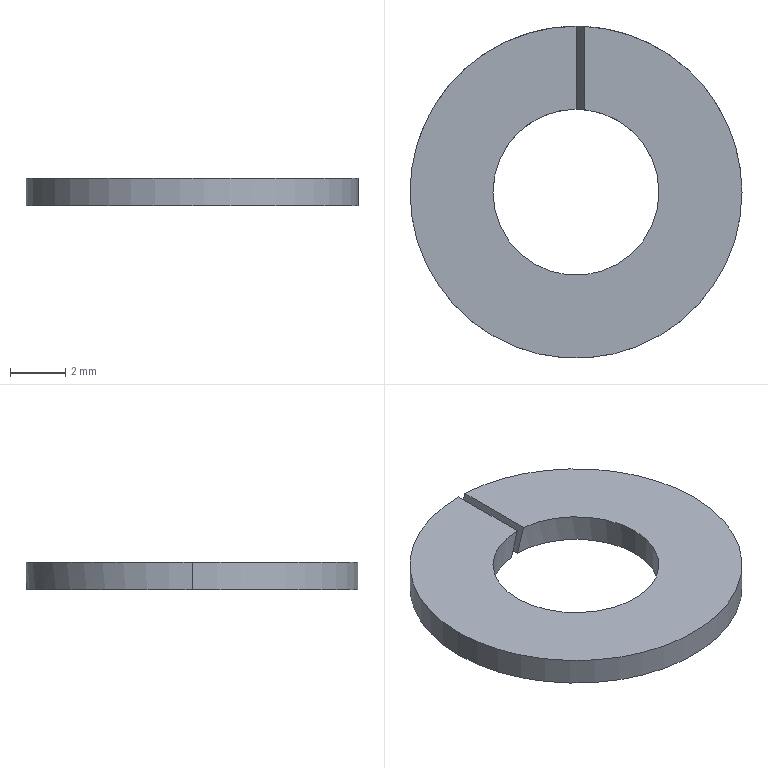Part | NX | features BREP 1 | 1 solid | 10 faces | box 12 x 12 x 1 mm | volume 83.879 mm3 | cylinder 6 | plane 4 | commonest cylinder face diameters 6 x3 12 x3
STEP:
#1=CARTESIAN_POINT('',(-3.,0.,-1.));
#2=VERTEX_POINT('',#1);
#3=CARTESIAN_POINT('',(3.,0.,-1.));
#4=VERTEX_POINT('',#3);
#5=CARTESIAN_POINT('',(0.,0.,-1.));
#6=DIRECTION('',(0.,0.,1.));
#7=DIRECTION('',(1.,0.,0.));
#8=AXIS2_PLACEMENT_3D('',#5,#6,#7);
#9=CIRCLE('',#8,3.);
#10=EDGE_CURVE('',#2,#4,#9,.T.);
#11=ORIENTED_EDGE('',*,*,#10,.F.);
#12=CARTESIAN_POINT('',(-3.,0.,0.));
#13=VERTEX_POINT('',#12);
#14=CARTESIAN_POINT('',(-3.,0.,-1.));
#15=DIRECTION('',(0.,0.,1.));
#16=VECTOR('',#15,1000.);
#17=LINE('',#14,#16);
#18=EDGE_CURVE('',#2,#13,#17,.T.);
#19=ORIENTED_EDGE('',*,*,#18,.T.);
#20=CARTESIAN_POINT('',(3.,0.,0.));
#21=VERTEX_POINT('',#20);
#22=CARTESIAN_POINT('',(0.,0.,0.));
#23=DIRECTION('',(0.,0.,1.));
#24=DIRECTION('',(1.,0.,0.));
#25=AXIS2_PLACEMENT_3D('',#22,#23,#24);
#26=CIRCLE('',#25,3.);
#27=EDGE_CURVE('',#13,#21,#26,.T.);
#28=ORIENTED_EDGE('',*,*,#27,.T.);
#29=CARTESIAN_POINT('',(3.,0.,-1.));
#30=DIRECTION('',(0.,0.,1.));
#31=VECTOR('',#30,1000.);
#32=LINE('',#29,#31);
#33=EDGE_CURVE('',#4,#21,#32,.T.);
#34=ORIENTED_EDGE('',*,*,#33,.F.);
#35=EDGE_LOOP('',(#11,#19,#28,#34));
#36=FACE_BOUND('',#35,.T.);
#37=CARTESIAN_POINT('',(0.,0.,-1.));
#38=DIRECTION('',(0.,0.,1.));
#39=DIRECTION('',(-1.,0.,0.));
#40=AXIS2_PLACEMENT_3D('',#37,#38,#39);
#41=CYLINDRICAL_SURFACE('',#40,3.);
#42=ADVANCED_FACE('',(#36),#41,.F.);
#43=CARTESIAN_POINT('',(0.,3.,-1.));
#44=VERTEX_POINT('',#43);
#45=CARTESIAN_POINT('',(0.,0.,-1.));
#46=DIRECTION('',(0.,0.,1.));
#47=DIRECTION('',(1.,0.,0.));
#48=AXIS2_PLACEMENT_3D('',#45,#46,#47);
#49=CIRCLE('',#48,3.);
#50=EDGE_CURVE('',#4,#44,#49,.T.);
#51=ORIENTED_EDGE('',*,*,#50,.F.);
#52=ORIENTED_EDGE('',*,*,#33,.T.);
#53=CARTESIAN_POINT('',(0.3145,2.983,0.));
#54=VERTEX_POINT('',#53);
#55=CARTESIAN_POINT('',(0.,0.,0.));
#56=DIRECTION('',(0.,0.,1.));
#57=DIRECTION('',(1.,0.,0.));
#58=AXIS2_PLACEMENT_3D('',#55,#56,#57);
#59=CIRCLE('',#58,3.);
#60=EDGE_CURVE('',#21,#54,#59,.T.);
#61=ORIENTED_EDGE('',*,*,#60,.T.);
#62=CARTESIAN_POINT('',(0.,3.,-1.));
#63=CARTESIAN_POINT('',(0.1051,3.,-0.6659));
#64=CARTESIAN_POINT('',(0.21,2.994,-0.3323));
#65=CARTESIAN_POINT('',(0.3145,2.983,0.));
#66=(BOUNDED_CURVE()B_SPLINE_CURVE(3,(#62,#63,#64,#65),.UNSPECIFIED.,.F.,.F.)B_SPLINE_CURVE_WITH_KNOTS((4,4),(0.,1.),.PIECEWISE_BEZIER_KNOTS.)CURVE()GEOMETRIC_REPRESENTATION_ITEM()RATIONAL_B_SPLINE_CURVE((1.,0.9991,0.9991,1.))REPRESENTATION_ITEM(''));
#67=EDGE_CURVE('',#44,#54,#66,.T.);
#68=ORIENTED_EDGE('',*,*,#67,.F.);
#69=EDGE_LOOP('',(#51,#52,#61,#68));
#70=FACE_BOUND('',#69,.T.);
#71=CARTESIAN_POINT('',(0.,0.,-1.));
#72=DIRECTION('',(0.,0.,1.));
#73=DIRECTION('',(-1.,0.,0.));
#74=AXIS2_PLACEMENT_3D('',#71,#72,#73);
#75=CYLINDRICAL_SURFACE('',#74,3.);
#76=ADVANCED_FACE('',(#70),#75,.F.);
#77=CARTESIAN_POINT('',(-0.3145,5.992,-1.));
#78=VERTEX_POINT('',#77);
#79=CARTESIAN_POINT('',(-6.,0.,-1.));
#80=VERTEX_POINT('',#79);
#81=CARTESIAN_POINT('',(0.,0.,-1.));
#82=DIRECTION('',(0.,0.,1.));
#83=DIRECTION('',(1.,0.,0.));
#84=AXIS2_PLACEMENT_3D('',#81,#82,#83);
#85=CIRCLE('',#84,6.);
#86=EDGE_CURVE('',#78,#80,#85,.T.);
#87=ORIENTED_EDGE('',*,*,#86,.T.);
#88=CARTESIAN_POINT('',(-6.,0.,0.));
#89=VERTEX_POINT('',#88);
#90=CARTESIAN_POINT('',(-6.,0.,-1.));
#91=DIRECTION('',(0.,0.,1.));
#92=VECTOR('',#91,1000.);
#93=LINE('',#90,#92);
#94=EDGE_CURVE('',#80,#89,#93,.T.);
#95=ORIENTED_EDGE('',*,*,#94,.T.);
#96=CARTESIAN_POINT('',(0.,6.,0.));
#97=VERTEX_POINT('',#96);
#98=CARTESIAN_POINT('',(0.,0.,0.));
#99=DIRECTION('',(0.,0.,1.));
#100=DIRECTION('',(1.,0.,0.));
#101=AXIS2_PLACEMENT_3D('',#98,#99,#100);
#102=CIRCLE('',#101,6.);
#103=EDGE_CURVE('',#97,#89,#102,.T.);
#104=ORIENTED_EDGE('',*,*,#103,.F.);
#105=CARTESIAN_POINT('',(0.,6.,0.));
#106=CARTESIAN_POINT('',(-0.1049,6.,-0.3335));
#107=CARTESIAN_POINT('',(-0.2097,5.997,-0.6669));
#108=CARTESIAN_POINT('',(-0.3145,5.992,-1.));
#109=(BOUNDED_CURVE()B_SPLINE_CURVE(3,(#105,#106,#107,#108),.UNSPECIFIED.,.F.,.F.)B_SPLINE_CURVE_WITH_KNOTS((4,4),(0.,1.),.PIECEWISE_BEZIER_KNOTS.)CURVE()GEOMETRIC_REPRESENTATION_ITEM()RATIONAL_B_SPLINE_CURVE((1.,0.9998,0.9998,1.))REPRESENTATION_ITEM(''));
#110=EDGE_CURVE('',#97,#78,#109,.T.);
#111=ORIENTED_EDGE('',*,*,#110,.T.);
#112=EDGE_LOOP('',(#87,#95,#104,#111));
#113=FACE_BOUND('',#112,.T.);
#114=CARTESIAN_POINT('',(0.,0.,-1.));
#115=DIRECTION('',(0.,0.,1.));
#116=DIRECTION('',(-1.,0.,0.));
#117=AXIS2_PLACEMENT_3D('',#114,#115,#116);
#118=CYLINDRICAL_SURFACE('',#117,6.);
#119=ADVANCED_FACE('',(#113),#118,.T.);
#120=ORIENTED_EDGE('',*,*,#94,.F.);
#121=CARTESIAN_POINT('',(6.,0.,-1.));
#122=VERTEX_POINT('',#121);
#123=CARTESIAN_POINT('',(0.,0.,-1.));
#124=DIRECTION('',(0.,0.,1.));
#125=DIRECTION('',(1.,0.,0.));
#126=AXIS2_PLACEMENT_3D('',#123,#124,#125);
#127=CIRCLE('',#126,6.);
#128=EDGE_CURVE('',#80,#122,#127,.T.);
#129=ORIENTED_EDGE('',*,*,#128,.T.);
#130=CARTESIAN_POINT('',(6.,0.,0.));
#131=VERTEX_POINT('',#130);
#132=CARTESIAN_POINT('',(6.,0.,-1.));
#133=DIRECTION('',(0.,0.,1.));
#134=VECTOR('',#133,1000.);
#135=LINE('',#132,#134);
#136=EDGE_CURVE('',#122,#131,#135,.T.);
#137=ORIENTED_EDGE('',*,*,#136,.T.);
#138=CARTESIAN_POINT('',(0.,0.,0.));
#139=DIRECTION('',(0.,0.,1.));
#140=DIRECTION('',(1.,0.,0.));
#141=AXIS2_PLACEMENT_3D('',#138,#139,#140);
#142=CIRCLE('',#141,6.);
#143=EDGE_CURVE('',#89,#131,#142,.T.);
#144=ORIENTED_EDGE('',*,*,#143,.F.);
#145=EDGE_LOOP('',(#120,#129,#137,#144));
#146=FACE_BOUND('',#145,.T.);
#147=CARTESIAN_POINT('',(0.,0.,-1.));
#148=DIRECTION('',(0.,0.,1.));
#149=DIRECTION('',(-1.,0.,0.));
#150=AXIS2_PLACEMENT_3D('',#147,#148,#149);
#151=CYLINDRICAL_SURFACE('',#150,6.);
#152=ADVANCED_FACE('',(#146),#151,.T.);
#153=ORIENTED_EDGE('',*,*,#136,.F.);
#154=CARTESIAN_POINT('',(0.,6.,-1.));
#155=VERTEX_POINT('',#154);
#156=CARTESIAN_POINT('',(0.,0.,-1.));
#157=DIRECTION('',(0.,0.,1.));
#158=DIRECTION('',(1.,0.,0.));
#159=AXIS2_PLACEMENT_3D('',#156,#157,#158);
#160=CIRCLE('',#159,6.);
#161=EDGE_CURVE('',#122,#155,#160,.T.);
#162=ORIENTED_EDGE('',*,*,#161,.T.);
#163=CARTESIAN_POINT('',(0.3145,5.992,0.));
#164=VERTEX_POINT('',#163);
#165=CARTESIAN_POINT('',(0.,6.,-1.));
#166=CARTESIAN_POINT('',(0.1049,6.,-0.6665));
#167=CARTESIAN_POINT('',(0.2097,5.997,-0.3331));
#168=CARTESIAN_POINT('',(0.3145,5.992,0.));
#169=(BOUNDED_CURVE()B_SPLINE_CURVE(3,(#165,#166,#167,#168),.UNSPECIFIED.,.F.,.F.)B_SPLINE_CURVE_WITH_KNOTS((4,4),(0.,1.),.PIECEWISE_BEZIER_KNOTS.)CURVE()GEOMETRIC_REPRESENTATION_ITEM()RATIONAL_B_SPLINE_CURVE((1.,0.9998,0.9998,1.))REPRESENTATION_ITEM(''));
#170=EDGE_CURVE('',#155,#164,#169,.T.);
#171=ORIENTED_EDGE('',*,*,#170,.T.);
#172=CARTESIAN_POINT('',(0.,0.,0.));
#173=DIRECTION('',(0.,0.,1.));
#174=DIRECTION('',(1.,0.,0.));
#175=AXIS2_PLACEMENT_3D('',#172,#173,#174);
#176=CIRCLE('',#175,6.);
#177=EDGE_CURVE('',#131,#164,#176,.T.);
#178=ORIENTED_EDGE('',*,*,#177,.F.);
#179=EDGE_LOOP('',(#153,#162,#171,#178));
#180=FACE_BOUND('',#179,.T.);
#181=CARTESIAN_POINT('',(0.,0.,-1.));
#182=DIRECTION('',(0.,0.,1.));
#183=DIRECTION('',(-1.,0.,0.));
#184=AXIS2_PLACEMENT_3D('',#181,#182,#183);
#185=CYLINDRICAL_SURFACE('',#184,6.);
#186=ADVANCED_FACE('',(#180),#185,.T.);
#187=CARTESIAN_POINT('',(-0.3145,2.983,-1.));
#188=VERTEX_POINT('',#187);
#189=CARTESIAN_POINT('',(-0.3145,6.,-1.));
#190=DIRECTION('',(0.,-1.,0.));
#191=VECTOR('',#190,1000.);
#192=LINE('',#189,#191);
#193=EDGE_CURVE('',#78,#188,#192,.T.);
#194=ORIENTED_EDGE('',*,*,#193,.T.);
#195=CARTESIAN_POINT('',(0.,0.,-1.));
#196=DIRECTION('',(0.,0.,1.));
#197=DIRECTION('',(1.,0.,0.));
#198=AXIS2_PLACEMENT_3D('',#195,#196,#197);
#199=CIRCLE('',#198,3.);
#200=EDGE_CURVE('',#188,#2,#199,.T.);
#201=ORIENTED_EDGE('',*,*,#200,.T.);
#202=ORIENTED_EDGE('',*,*,#10,.T.);
#203=ORIENTED_EDGE('',*,*,#50,.T.);
#204=CARTESIAN_POINT('',(0.,6.,-1.));
#205=DIRECTION('',(0.,-1.,0.));
#206=VECTOR('',#205,1000.);
#207=LINE('',#204,#206);
#208=EDGE_CURVE('',#155,#44,#207,.T.);
#209=ORIENTED_EDGE('',*,*,#208,.F.);
#210=ORIENTED_EDGE('',*,*,#161,.F.);
#211=ORIENTED_EDGE('',*,*,#128,.F.);
#212=ORIENTED_EDGE('',*,*,#86,.F.);
#213=EDGE_LOOP('',(#194,#201,#202,#203,#209,#210,#211,#212));
#214=FACE_BOUND('',#213,.T.);
#215=CARTESIAN_POINT('',(0.,0.,-1.));
#216=DIRECTION('',(0.,0.,1.));
#217=DIRECTION('',(-1.,0.,0.));
#218=AXIS2_PLACEMENT_3D('',#215,#216,#217);
#219=PLANE('',#218);
#220=ADVANCED_FACE('',(#214),#219,.F.);
#221=CARTESIAN_POINT('',(0.,3.,0.));
#222=VERTEX_POINT('',#221);
#223=CARTESIAN_POINT('',(0.,0.,0.));
#224=DIRECTION('',(0.,0.,1.));
#225=DIRECTION('',(1.,0.,0.));
#226=AXIS2_PLACEMENT_3D('',#223,#224,#225);
#227=CIRCLE('',#226,3.);
#228=EDGE_CURVE('',#222,#13,#227,.T.);
#229=ORIENTED_EDGE('',*,*,#228,.F.);
#230=CARTESIAN_POINT('',(0.,6.,0.));
#231=DIRECTION('',(0.,-1.,0.));
#232=VECTOR('',#231,1000.);
#233=LINE('',#230,#232);
#234=EDGE_CURVE('',#97,#222,#233,.T.);
#235=ORIENTED_EDGE('',*,*,#234,.F.);
#236=ORIENTED_EDGE('',*,*,#103,.T.);
#237=ORIENTED_EDGE('',*,*,#143,.T.);
#238=ORIENTED_EDGE('',*,*,#177,.T.);
#239=CARTESIAN_POINT('',(0.3145,6.,0.));
#240=DIRECTION('',(0.,-1.,0.));
#241=VECTOR('',#240,1000.);
#242=LINE('',#239,#241);
#243=EDGE_CURVE('',#164,#54,#242,.T.);
#244=ORIENTED_EDGE('',*,*,#243,.T.);
#245=ORIENTED_EDGE('',*,*,#60,.F.);
#246=ORIENTED_EDGE('',*,*,#27,.F.);
#247=EDGE_LOOP('',(#229,#235,#236,#237,#238,#244,#245,#246));
#248=FACE_BOUND('',#247,.T.);
#249=CARTESIAN_POINT('',(0.,0.,0.));
#250=DIRECTION('',(0.,0.,1.));
#251=DIRECTION('',(-1.,0.,0.));
#252=AXIS2_PLACEMENT_3D('',#249,#250,#251);
#253=PLANE('',#252);
#254=ADVANCED_FACE('',(#248),#253,.T.);
#255=ORIENTED_EDGE('',*,*,#18,.F.);
#256=ORIENTED_EDGE('',*,*,#200,.F.);
#257=CARTESIAN_POINT('',(0.,3.,0.));
#258=CARTESIAN_POINT('',(-0.1051,3.,-0.3341));
#259=CARTESIAN_POINT('',(-0.21,2.994,-0.6677));
#260=CARTESIAN_POINT('',(-0.3145,2.983,-1.));
#261=(BOUNDED_CURVE()B_SPLINE_CURVE(3,(#257,#258,#259,#260),.UNSPECIFIED.,.F.,.F.)B_SPLINE_CURVE_WITH_KNOTS((4,4),(0.,1.),.PIECEWISE_BEZIER_KNOTS.)CURVE()GEOMETRIC_REPRESENTATION_ITEM()RATIONAL_B_SPLINE_CURVE((1.,0.9991,0.9991,1.))REPRESENTATION_ITEM(''));
#262=EDGE_CURVE('',#222,#188,#261,.T.);
#263=ORIENTED_EDGE('',*,*,#262,.F.);
#264=ORIENTED_EDGE('',*,*,#228,.T.);
#265=EDGE_LOOP('',(#255,#256,#263,#264));
#266=FACE_BOUND('',#265,.T.);
#267=CARTESIAN_POINT('',(0.,0.,-1.));
#268=DIRECTION('',(0.,0.,1.));
#269=DIRECTION('',(-1.,0.,0.));
#270=AXIS2_PLACEMENT_3D('',#267,#268,#269);
#271=CYLINDRICAL_SURFACE('',#270,3.);
#272=ADVANCED_FACE('',(#266),#271,.F.);
#273=ORIENTED_EDGE('',*,*,#208,.T.);
#274=ORIENTED_EDGE('',*,*,#67,.T.);
#275=ORIENTED_EDGE('',*,*,#243,.F.);
#276=ORIENTED_EDGE('',*,*,#170,.F.);
#277=EDGE_LOOP('',(#273,#274,#275,#276));
#278=FACE_BOUND('',#277,.T.);
#279=CARTESIAN_POINT('',(0.,6.,-1.));
#280=DIRECTION('',(-0.9539,0.,0.3));
#281=DIRECTION('',(0.,-1.,0.));
#282=AXIS2_PLACEMENT_3D('',#279,#280,#281);
#283=PLANE('',#282);
#284=ADVANCED_FACE('',(#278),#283,.T.);
#285=ORIENTED_EDGE('',*,*,#234,.T.);
#286=ORIENTED_EDGE('',*,*,#262,.T.);
#287=ORIENTED_EDGE('',*,*,#193,.F.);
#288=ORIENTED_EDGE('',*,*,#110,.F.);
#289=EDGE_LOOP('',(#285,#286,#287,#288));
#290=FACE_BOUND('',#289,.T.);
#291=CARTESIAN_POINT('',(0.,6.,0.));
#292=DIRECTION('',(0.9539,0.,-0.3));
#293=DIRECTION('',(0.,1.,0.));
#294=AXIS2_PLACEMENT_3D('',#291,#292,#293);
#295=PLANE('',#294);
#296=ADVANCED_FACE('',(#290),#295,.T.);
#297=CLOSED_SHELL('',(#42,#76,#119,#152,#186,#220,#254,#272,#284,#296));
#298=MANIFOLD_SOLID_BREP('',#297);
#299=(LENGTH_UNIT()NAMED_UNIT(*)SI_UNIT(.MILLI.,.METRE.));
#300=UNCERTAINTY_MEASURE_WITH_UNIT(LENGTH_MEASURE(0.00001),#299,'','');
#301=(NAMED_UNIT(*)PLANE_ANGLE_UNIT()SI_UNIT($,.RADIAN.));
#302=(NAMED_UNIT(*)SI_UNIT($,.STERADIAN.)SOLID_ANGLE_UNIT());
#303=(GEOMETRIC_REPRESENTATION_CONTEXT(3)GLOBAL_UNCERTAINTY_ASSIGNED_CONTEXT((#300))GLOBAL_UNIT_ASSIGNED_CONTEXT((#299,#301,#302))REPRESENTATION_CONTEXT('',''));
#304=ADVANCED_BREP_SHAPE_REPRESENTATION('',(#298),#303);